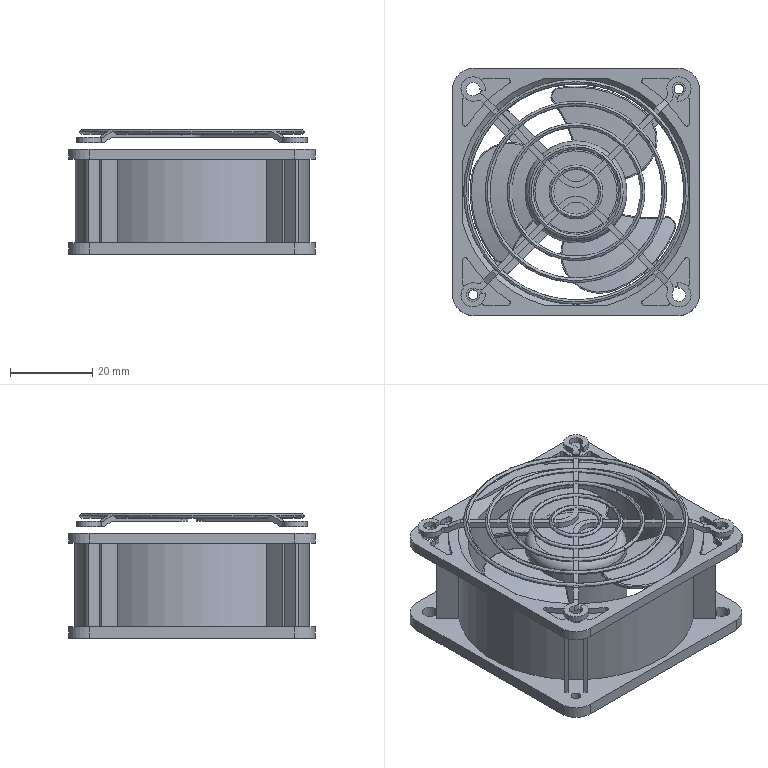Part | NX | features BREP 3 | 2 solids | 384 faces | box 60 x 60 x 30.335 mm | volume 28781 mm3 | plane 157 | cylinder 119 | spline 52 | torus 51 | cone 5 | commonest cylinder face diameters 1.429 x32 4.762 x14 10 x8 57.143 x8 61.905 x8 2.381 x4